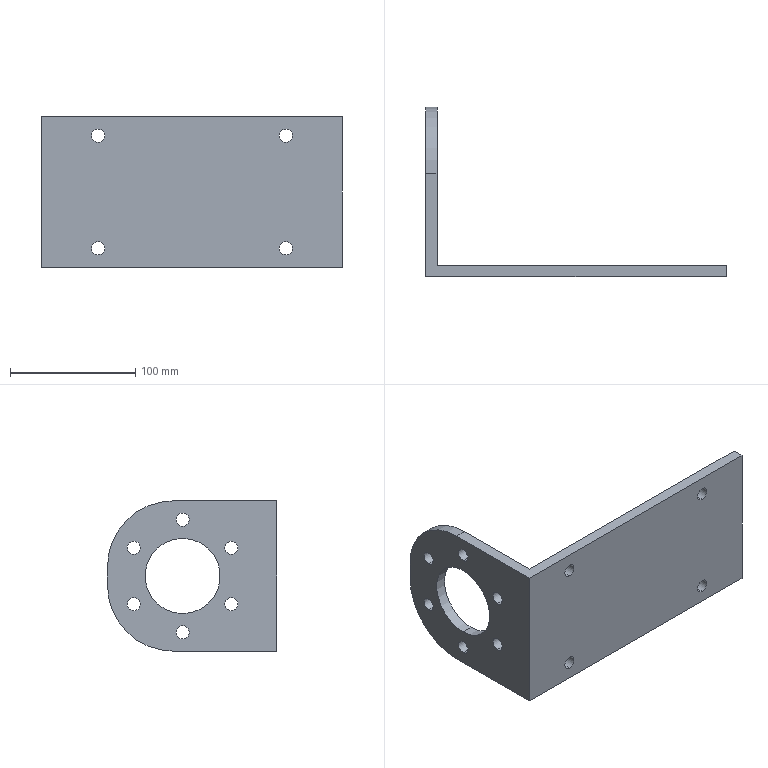Part | SolidWorks | features ICE 3, BaseBody 1 | 1 solid | 32 faces | box 240 x 135 x 120 mm | volume 351393 mm3 | cylinder 24 | plane 8 | commonest cylinder face diameters 10.5 x20 60 x2 105 x2
STEP:
#1=CARTESIAN_POINT('',(195.,9.,-39.75));
#2=VERTEX_POINT('',#1);
#3=CARTESIAN_POINT('',(195.,9.,-50.25));
#4=VERTEX_POINT('',#3);
#5=CARTESIAN_POINT('',(195.,9.,-45.));
#6=DIRECTION('',(0.,-1.,0.));
#7=DIRECTION('',(0.,0.,-1.));
#8=AXIS2_PLACEMENT_3D('',#5,#6,#7);
#9=CIRCLE('',#8,5.25);
#10=EDGE_CURVE('',#2,#4,#9,.T.);
#11=ORIENTED_EDGE('',*,*,#10,.F.);
#12=CARTESIAN_POINT('',(195.,0.,-39.75));
#13=VERTEX_POINT('',#12);
#14=CARTESIAN_POINT('',(195.,135.,-39.75));
#15=DIRECTION('',(0.,-1.,0.));
#16=VECTOR('',#15,1000.);
#17=LINE('',#14,#16);
#18=EDGE_CURVE('',#2,#13,#17,.T.);
#19=ORIENTED_EDGE('',*,*,#18,.T.);
#20=CARTESIAN_POINT('',(195.,0.,-50.25));
#21=VERTEX_POINT('',#20);
#22=CARTESIAN_POINT('',(195.,0.,-45.));
#23=DIRECTION('',(0.,-1.,0.));
#24=DIRECTION('',(0.,0.,-1.));
#25=AXIS2_PLACEMENT_3D('',#22,#23,#24);
#26=CIRCLE('',#25,5.25);
#27=EDGE_CURVE('',#13,#21,#26,.T.);
#28=ORIENTED_EDGE('',*,*,#27,.T.);
#29=CARTESIAN_POINT('',(195.,135.,-50.25));
#30=DIRECTION('',(0.,-1.,0.));
#31=VECTOR('',#30,1000.);
#32=LINE('',#29,#31);
#33=EDGE_CURVE('',#4,#21,#32,.T.);
#34=ORIENTED_EDGE('',*,*,#33,.F.);
#35=EDGE_LOOP('',(#11,#19,#28,#34));
#36=FACE_OUTER_BOUND('',#35,.T.);
#37=CARTESIAN_POINT('',(195.,135.,-45.));
#38=DIRECTION('',(0.,-1.,0.));
#39=DIRECTION('',(0.,0.,-1.));
#40=AXIS2_PLACEMENT_3D('',#37,#38,#39);
#41=CYLINDRICAL_SURFACE('',#40,5.25);
#42=ADVANCED_FACE('',(#36),#41,.F.);
#43=CARTESIAN_POINT('',(45.,9.,-39.75));
#44=VERTEX_POINT('',#43);
#45=CARTESIAN_POINT('',(45.,9.,-50.25));
#46=VERTEX_POINT('',#45);
#47=CARTESIAN_POINT('',(45.,9.,-45.));
#48=DIRECTION('',(0.,-1.,0.));
#49=DIRECTION('',(0.,0.,-1.));
#50=AXIS2_PLACEMENT_3D('',#47,#48,#49);
#51=CIRCLE('',#50,5.25);
#52=EDGE_CURVE('',#44,#46,#51,.T.);
#53=ORIENTED_EDGE('',*,*,#52,.F.);
#54=CARTESIAN_POINT('',(45.,0.,-39.75));
#55=VERTEX_POINT('',#54);
#56=CARTESIAN_POINT('',(45.,135.,-39.75));
#57=DIRECTION('',(0.,-1.,0.));
#58=VECTOR('',#57,1000.);
#59=LINE('',#56,#58);
#60=EDGE_CURVE('',#44,#55,#59,.T.);
#61=ORIENTED_EDGE('',*,*,#60,.T.);
#62=CARTESIAN_POINT('',(45.,0.,-50.25));
#63=VERTEX_POINT('',#62);
#64=CARTESIAN_POINT('',(45.,0.,-45.));
#65=DIRECTION('',(0.,-1.,0.));
#66=DIRECTION('',(0.,0.,-1.));
#67=AXIS2_PLACEMENT_3D('',#64,#65,#66);
#68=CIRCLE('',#67,5.25);
#69=EDGE_CURVE('',#55,#63,#68,.T.);
#70=ORIENTED_EDGE('',*,*,#69,.T.);
#71=CARTESIAN_POINT('',(45.,135.,-50.25));
#72=DIRECTION('',(0.,-1.,0.));
#73=VECTOR('',#72,1000.);
#74=LINE('',#71,#73);
#75=EDGE_CURVE('',#46,#63,#74,.T.);
#76=ORIENTED_EDGE('',*,*,#75,.F.);
#77=EDGE_LOOP('',(#53,#61,#70,#76));
#78=FACE_OUTER_BOUND('',#77,.T.);
#79=CARTESIAN_POINT('',(45.,135.,-45.));
#80=DIRECTION('',(0.,-1.,0.));
#81=DIRECTION('',(0.,0.,-1.));
#82=AXIS2_PLACEMENT_3D('',#79,#80,#81);
#83=CYLINDRICAL_SURFACE('',#82,5.25);
#84=ADVANCED_FACE('',(#78),#83,.F.);
#85=CARTESIAN_POINT('',(45.,9.,50.25));
#86=VERTEX_POINT('',#85);
#87=CARTESIAN_POINT('',(45.,9.,39.75));
#88=VERTEX_POINT('',#87);
#89=CARTESIAN_POINT('',(45.,9.,45.));
#90=DIRECTION('',(0.,-1.,0.));
#91=DIRECTION('',(0.,0.,-1.));
#92=AXIS2_PLACEMENT_3D('',#89,#90,#91);
#93=CIRCLE('',#92,5.25);
#94=EDGE_CURVE('',#86,#88,#93,.T.);
#95=ORIENTED_EDGE('',*,*,#94,.F.);
#96=CARTESIAN_POINT('',(45.,0.,50.25));
#97=VERTEX_POINT('',#96);
#98=CARTESIAN_POINT('',(45.,135.,50.25));
#99=DIRECTION('',(0.,-1.,0.));
#100=VECTOR('',#99,1000.);
#101=LINE('',#98,#100);
#102=EDGE_CURVE('',#86,#97,#101,.T.);
#103=ORIENTED_EDGE('',*,*,#102,.T.);
#104=CARTESIAN_POINT('',(45.,0.,39.75));
#105=VERTEX_POINT('',#104);
#106=CARTESIAN_POINT('',(45.,0.,45.));
#107=DIRECTION('',(0.,-1.,0.));
#108=DIRECTION('',(0.,0.,-1.));
#109=AXIS2_PLACEMENT_3D('',#106,#107,#108);
#110=CIRCLE('',#109,5.25);
#111=EDGE_CURVE('',#97,#105,#110,.T.);
#112=ORIENTED_EDGE('',*,*,#111,.T.);
#113=CARTESIAN_POINT('',(45.,135.,39.75));
#114=DIRECTION('',(0.,-1.,0.));
#115=VECTOR('',#114,1000.);
#116=LINE('',#113,#115);
#117=EDGE_CURVE('',#88,#105,#116,.T.);
#118=ORIENTED_EDGE('',*,*,#117,.F.);
#119=EDGE_LOOP('',(#95,#103,#112,#118));
#120=FACE_OUTER_BOUND('',#119,.T.);
#121=CARTESIAN_POINT('',(45.,135.,45.));
#122=DIRECTION('',(0.,-1.,0.));
#123=DIRECTION('',(0.,0.,-1.));
#124=AXIS2_PLACEMENT_3D('',#121,#122,#123);
#125=CYLINDRICAL_SURFACE('',#124,5.25);
#126=ADVANCED_FACE('',(#120),#125,.F.);
#127=CARTESIAN_POINT('',(195.,9.,50.25));
#128=VERTEX_POINT('',#127);
#129=CARTESIAN_POINT('',(195.,9.,39.75));
#130=VERTEX_POINT('',#129);
#131=CARTESIAN_POINT('',(195.,9.,45.));
#132=DIRECTION('',(0.,-1.,0.));
#133=DIRECTION('',(0.,0.,-1.));
#134=AXIS2_PLACEMENT_3D('',#131,#132,#133);
#135=CIRCLE('',#134,5.25);
#136=EDGE_CURVE('',#128,#130,#135,.T.);
#137=ORIENTED_EDGE('',*,*,#136,.F.);
#138=CARTESIAN_POINT('',(195.,0.,50.25));
#139=VERTEX_POINT('',#138);
#140=CARTESIAN_POINT('',(195.,135.,50.25));
#141=DIRECTION('',(0.,-1.,0.));
#142=VECTOR('',#141,1000.);
#143=LINE('',#140,#142);
#144=EDGE_CURVE('',#128,#139,#143,.T.);
#145=ORIENTED_EDGE('',*,*,#144,.T.);
#146=CARTESIAN_POINT('',(195.,0.,39.75));
#147=VERTEX_POINT('',#146);
#148=CARTESIAN_POINT('',(195.,0.,45.));
#149=DIRECTION('',(0.,-1.,0.));
#150=DIRECTION('',(0.,0.,-1.));
#151=AXIS2_PLACEMENT_3D('',#148,#149,#150);
#152=CIRCLE('',#151,5.25);
#153=EDGE_CURVE('',#139,#147,#152,.T.);
#154=ORIENTED_EDGE('',*,*,#153,.T.);
#155=CARTESIAN_POINT('',(195.,135.,39.75));
#156=DIRECTION('',(0.,-1.,0.));
#157=VECTOR('',#156,1000.);
#158=LINE('',#155,#157);
#159=EDGE_CURVE('',#130,#147,#158,.T.);
#160=ORIENTED_EDGE('',*,*,#159,.F.);
#161=EDGE_LOOP('',(#137,#145,#154,#160));
#162=FACE_OUTER_BOUND('',#161,.T.);
#163=CARTESIAN_POINT('',(195.,135.,45.));
#164=DIRECTION('',(0.,-1.,0.));
#165=DIRECTION('',(0.,0.,-1.));
#166=AXIS2_PLACEMENT_3D('',#163,#164,#165);
#167=CYLINDRICAL_SURFACE('',#166,5.25);
#168=ADVANCED_FACE('',(#162),#167,.F.);
#169=CARTESIAN_POINT('',(9.,75.,30.));
#170=VERTEX_POINT('',#169);
#171=CARTESIAN_POINT('',(9.,75.,-30.));
#172=VERTEX_POINT('',#171);
#173=CARTESIAN_POINT('',(9.,75.,0.));
#174=DIRECTION('',(1.,0.,0.));
#175=DIRECTION('',(0.,0.,1.));
#176=AXIS2_PLACEMENT_3D('',#173,#174,#175);
#177=CIRCLE('',#176,30.);
#178=EDGE_CURVE('',#170,#172,#177,.T.);
#179=ORIENTED_EDGE('',*,*,#178,.T.);
#180=CARTESIAN_POINT('',(0.,75.,-30.));
#181=VERTEX_POINT('',#180);
#182=CARTESIAN_POINT('',(9.,75.,-30.));
#183=DIRECTION('',(-1.,0.,0.));
#184=VECTOR('',#183,1000.);
#185=LINE('',#182,#184);
#186=EDGE_CURVE('',#172,#181,#185,.T.);
#187=ORIENTED_EDGE('',*,*,#186,.T.);
#188=CARTESIAN_POINT('',(0.,75.,30.));
#189=VERTEX_POINT('',#188);
#190=CARTESIAN_POINT('',(0.,75.,0.));
#191=DIRECTION('',(1.,0.,0.));
#192=DIRECTION('',(0.,0.,1.));
#193=AXIS2_PLACEMENT_3D('',#190,#191,#192);
#194=CIRCLE('',#193,30.);
#195=EDGE_CURVE('',#189,#181,#194,.T.);
#196=ORIENTED_EDGE('',*,*,#195,.F.);
#197=CARTESIAN_POINT('',(9.,75.,30.));
#198=DIRECTION('',(-1.,0.,0.));
#199=VECTOR('',#198,1000.);
#200=LINE('',#197,#199);
#201=EDGE_CURVE('',#170,#189,#200,.T.);
#202=ORIENTED_EDGE('',*,*,#201,.F.);
#203=EDGE_LOOP('',(#179,#187,#196,#202));
#204=FACE_OUTER_BOUND('',#203,.T.);
#205=CARTESIAN_POINT('',(9.,75.,0.));
#206=DIRECTION('',(-1.,0.,0.));
#207=DIRECTION('',(0.,0.,1.));
#208=AXIS2_PLACEMENT_3D('',#205,#206,#207);
#209=CYLINDRICAL_SURFACE('',#208,30.);
#210=ADVANCED_FACE('',(#204),#209,.F.);
#211=CARTESIAN_POINT('',(9.,75.,50.25));
#212=VERTEX_POINT('',#211);
#213=CARTESIAN_POINT('',(9.,75.,39.75));
#214=VERTEX_POINT('',#213);
#215=CARTESIAN_POINT('',(9.,75.,45.));
#216=DIRECTION('',(1.,0.,0.));
#217=DIRECTION('',(0.,0.,1.));
#218=AXIS2_PLACEMENT_3D('',#215,#216,#217);
#219=CIRCLE('',#218,5.25);
#220=EDGE_CURVE('',#212,#214,#219,.T.);
#221=ORIENTED_EDGE('',*,*,#220,.T.);
#222=CARTESIAN_POINT('',(0.,75.,39.75));
#223=VERTEX_POINT('',#222);
#224=CARTESIAN_POINT('',(9.,75.,39.75));
#225=DIRECTION('',(-1.,0.,0.));
#226=VECTOR('',#225,1000.);
#227=LINE('',#224,#226);
#228=EDGE_CURVE('',#214,#223,#227,.T.);
#229=ORIENTED_EDGE('',*,*,#228,.T.);
#230=CARTESIAN_POINT('',(0.,75.,50.25));
#231=VERTEX_POINT('',#230);
#232=CARTESIAN_POINT('',(0.,75.,45.));
#233=DIRECTION('',(1.,0.,0.));
#234=DIRECTION('',(0.,0.,1.));
#235=AXIS2_PLACEMENT_3D('',#232,#233,#234);
#236=CIRCLE('',#235,5.25);
#237=EDGE_CURVE('',#231,#223,#236,.T.);
#238=ORIENTED_EDGE('',*,*,#237,.F.);
#239=CARTESIAN_POINT('',(9.,75.,50.25));
#240=DIRECTION('',(-1.,0.,0.));
#241=VECTOR('',#240,1000.);
#242=LINE('',#239,#241);
#243=EDGE_CURVE('',#212,#231,#242,.T.);
#244=ORIENTED_EDGE('',*,*,#243,.F.);
#245=EDGE_LOOP('',(#221,#229,#238,#244));
#246=FACE_OUTER_BOUND('',#245,.T.);
#247=CARTESIAN_POINT('',(9.,75.,45.));
#248=DIRECTION('',(-1.,0.,0.));
#249=DIRECTION('',(0.,0.,1.));
#250=AXIS2_PLACEMENT_3D('',#247,#248,#249);
#251=CYLINDRICAL_SURFACE('',#250,5.25);
#252=ADVANCED_FACE('',(#246),#251,.F.);
#253=CARTESIAN_POINT('',(9.,113.971,27.75));
#254=VERTEX_POINT('',#253);
#255=CARTESIAN_POINT('',(9.,113.971,17.25));
#256=VERTEX_POINT('',#255);
#257=CARTESIAN_POINT('',(9.,113.971,22.5));
#258=DIRECTION('',(1.,0.,0.));
#259=DIRECTION('',(0.,0.,1.));
#260=AXIS2_PLACEMENT_3D('',#257,#258,#259);
#261=CIRCLE('',#260,5.25);
#262=EDGE_CURVE('',#254,#256,#261,.T.);
#263=ORIENTED_EDGE('',*,*,#262,.T.);
#264=CARTESIAN_POINT('',(0.,113.971,17.25));
#265=VERTEX_POINT('',#264);
#266=CARTESIAN_POINT('',(9.,113.971,17.25));
#267=DIRECTION('',(-1.,0.,0.));
#268=VECTOR('',#267,1000.);
#269=LINE('',#266,#268);
#270=EDGE_CURVE('',#256,#265,#269,.T.);
#271=ORIENTED_EDGE('',*,*,#270,.T.);
#272=CARTESIAN_POINT('',(0.,113.971,27.75));
#273=VERTEX_POINT('',#272);
#274=CARTESIAN_POINT('',(0.,113.971,22.5));
#275=DIRECTION('',(1.,0.,0.));
#276=DIRECTION('',(0.,0.,1.));
#277=AXIS2_PLACEMENT_3D('',#274,#275,#276);
#278=CIRCLE('',#277,5.25);
#279=EDGE_CURVE('',#273,#265,#278,.T.);
#280=ORIENTED_EDGE('',*,*,#279,.F.);
#281=CARTESIAN_POINT('',(9.,113.971,27.75));
#282=DIRECTION('',(-1.,0.,0.));
#283=VECTOR('',#282,1000.);
#284=LINE('',#281,#283);
#285=EDGE_CURVE('',#254,#273,#284,.T.);
#286=ORIENTED_EDGE('',*,*,#285,.F.);
#287=EDGE_LOOP('',(#263,#271,#280,#286));
#288=FACE_OUTER_BOUND('',#287,.T.);
#289=CARTESIAN_POINT('',(9.,113.971,22.5));
#290=DIRECTION('',(-1.,0.,0.));
#291=DIRECTION('',(0.,0.,1.));
#292=AXIS2_PLACEMENT_3D('',#289,#290,#291);
#293=CYLINDRICAL_SURFACE('',#292,5.25);
#294=ADVANCED_FACE('',(#288),#293,.F.);
#295=CARTESIAN_POINT('',(9.,113.971,-17.25));
#296=VERTEX_POINT('',#295);
#297=CARTESIAN_POINT('',(9.,113.971,-27.75));
#298=VERTEX_POINT('',#297);
#299=CARTESIAN_POINT('',(9.,113.971,-22.5));
#300=DIRECTION('',(1.,0.,0.));
#301=DIRECTION('',(0.,0.,1.));
#302=AXIS2_PLACEMENT_3D('',#299,#300,#301);
#303=CIRCLE('',#302,5.25);
#304=EDGE_CURVE('',#296,#298,#303,.T.);
#305=ORIENTED_EDGE('',*,*,#304,.T.);
#306=CARTESIAN_POINT('',(0.,113.971,-27.75));
#307=VERTEX_POINT('',#306);
#308=CARTESIAN_POINT('',(9.,113.971,-27.75));
#309=DIRECTION('',(-1.,0.,0.));
#310=VECTOR('',#309,1000.);
#311=LINE('',#308,#310);
#312=EDGE_CURVE('',#298,#307,#311,.T.);
#313=ORIENTED_EDGE('',*,*,#312,.T.);
#314=CARTESIAN_POINT('',(0.,113.971,-17.25));
#315=VERTEX_POINT('',#314);
#316=CARTESIAN_POINT('',(0.,113.971,-22.5));
#317=DIRECTION('',(1.,0.,0.));
#318=DIRECTION('',(0.,0.,1.));
#319=AXIS2_PLACEMENT_3D('',#316,#317,#318);
#320=CIRCLE('',#319,5.25);
#321=EDGE_CURVE('',#315,#307,#320,.T.);
#322=ORIENTED_EDGE('',*,*,#321,.F.);
#323=CARTESIAN_POINT('',(9.,113.971,-17.25));
#324=DIRECTION('',(-1.,0.,0.));
#325=VECTOR('',#324,1000.);
#326=LINE('',#323,#325);
#327=EDGE_CURVE('',#296,#315,#326,.T.);
#328=ORIENTED_EDGE('',*,*,#327,.F.);
#329=EDGE_LOOP('',(#305,#313,#322,#328));
#330=FACE_OUTER_BOUND('',#329,.T.);
#331=CARTESIAN_POINT('',(9.,113.971,-22.5));
#332=DIRECTION('',(-1.,0.,0.));
#333=DIRECTION('',(0.,0.,1.));
#334=AXIS2_PLACEMENT_3D('',#331,#332,#333);
#335=CYLINDRICAL_SURFACE('',#334,5.25);
#336=ADVANCED_FACE('',(#330),#335,.F.);
#337=CARTESIAN_POINT('',(9.,75.,-39.75));
#338=VERTEX_POINT('',#337);
#339=CARTESIAN_POINT('',(9.,75.,-50.25));
#340=VERTEX_POINT('',#339);
#341=CARTESIAN_POINT('',(9.,75.,-45.));
#342=DIRECTION('',(1.,0.,0.));
#343=DIRECTION('',(0.,0.,1.));
#344=AXIS2_PLACEMENT_3D('',#341,#342,#343);
#345=CIRCLE('',#344,5.25);
#346=EDGE_CURVE('',#338,#340,#345,.T.);
#347=ORIENTED_EDGE('',*,*,#346,.T.);
#348=CARTESIAN_POINT('',(0.,75.,-50.25));
#349=VERTEX_POINT('',#348);
#350=CARTESIAN_POINT('',(9.,75.,-50.25));
#351=DIRECTION('',(-1.,0.,0.));
#352=VECTOR('',#351,1000.);
#353=LINE('',#350,#352);
#354=EDGE_CURVE('',#340,#349,#353,.T.);
#355=ORIENTED_EDGE('',*,*,#354,.T.);
#356=CARTESIAN_POINT('',(0.,75.,-39.75));
#357=VERTEX_POINT('',#356);
#358=CARTESIAN_POINT('',(0.,75.,-45.));
#359=DIRECTION('',(1.,0.,0.));
#360=DIRECTION('',(0.,0.,1.));
#361=AXIS2_PLACEMENT_3D('',#358,#359,#360);
#362=CIRCLE('',#361,5.25);
#363=EDGE_CURVE('',#357,#349,#362,.T.);
#364=ORIENTED_EDGE('',*,*,#363,.F.);
#365=CARTESIAN_POINT('',(9.,75.,-39.75));
#366=DIRECTION('',(-1.,0.,0.));
#367=VECTOR('',#366,1000.);
#368=LINE('',#365,#367);
#369=EDGE_CURVE('',#338,#357,#368,.T.);
#370=ORIENTED_EDGE('',*,*,#369,.F.);
#371=EDGE_LOOP('',(#347,#355,#364,#370));
#372=FACE_OUTER_BOUND('',#371,.T.);
#373=CARTESIAN_POINT('',(9.,75.,-45.));
#374=DIRECTION('',(-1.,0.,0.));
#375=DIRECTION('',(0.,0.,1.));
#376=AXIS2_PLACEMENT_3D('',#373,#374,#375);
#377=CYLINDRICAL_SURFACE('',#376,5.25);
#378=ADVANCED_FACE('',(#372),#377,.F.);
#379=CARTESIAN_POINT('',(9.,36.029,-17.25));
#380=VERTEX_POINT('',#379);
#381=CARTESIAN_POINT('',(9.,36.029,-27.75));
#382=VERTEX_POINT('',#381);
#383=CARTESIAN_POINT('',(9.,36.029,-22.5));
#384=DIRECTION('',(1.,0.,0.));
#385=DIRECTION('',(0.,0.,1.));
#386=AXIS2_PLACEMENT_3D('',#383,#384,#385);
#387=CIRCLE('',#386,5.25);
#388=EDGE_CURVE('',#380,#382,#387,.T.);
#389=ORIENTED_EDGE('',*,*,#388,.T.);
#390=CARTESIAN_POINT('',(0.,36.029,-27.75));
#391=VERTEX_POINT('',#390);
#392=CARTESIAN_POINT('',(9.,36.029,-27.75));
#393=DIRECTION('',(-1.,0.,0.));
#394=VECTOR('',#393,1000.);
#395=LINE('',#392,#394);
#396=EDGE_CURVE('',#382,#391,#395,.T.);
#397=ORIENTED_EDGE('',*,*,#396,.T.);
#398=CARTESIAN_POINT('',(0.,36.029,-17.25));
#399=VERTEX_POINT('',#398);
#400=CARTESIAN_POINT('',(0.,36.029,-22.5));
#401=DIRECTION('',(1.,0.,0.));
#402=DIRECTION('',(0.,0.,1.));
#403=AXIS2_PLACEMENT_3D('',#400,#401,#402);
#404=CIRCLE('',#403,5.25);
#405=EDGE_CURVE('',#399,#391,#404,.T.);
#406=ORIENTED_EDGE('',*,*,#405,.F.);
#407=CARTESIAN_POINT('',(9.,36.029,-17.25));
#408=DIRECTION('',(-1.,0.,0.));
#409=VECTOR('',#408,1000.);
#410=LINE('',#407,#409);
#411=EDGE_CURVE('',#380,#399,#410,.T.);
#412=ORIENTED_EDGE('',*,*,#411,.F.);
#413=EDGE_LOOP('',(#389,#397,#406,#412));
#414=FACE_OUTER_BOUND('',#413,.T.);
#415=CARTESIAN_POINT('',(9.,36.029,-22.5));
#416=DIRECTION('',(-1.,0.,0.));
#417=DIRECTION('',(0.,0.,1.));
#418=AXIS2_PLACEMENT_3D('',#415,#416,#417);
#419=CYLINDRICAL_SURFACE('',#418,5.25);
#420=ADVANCED_FACE('',(#414),#419,.F.);
#421=CARTESIAN_POINT('',(9.,36.029,27.75));
#422=VERTEX_POINT('',#421);
#423=CARTESIAN_POINT('',(9.,36.029,17.25));
#424=VERTEX_POINT('',#423);
#425=CARTESIAN_POINT('',(9.,36.029,22.5));
#426=DIRECTION('',(1.,0.,0.));
#427=DIRECTION('',(0.,0.,1.));
#428=AXIS2_PLACEMENT_3D('',#425,#426,#427);
#429=CIRCLE('',#428,5.25);
#430=EDGE_CURVE('',#422,#424,#429,.T.);
#431=ORIENTED_EDGE('',*,*,#430,.T.);
#432=CARTESIAN_POINT('',(0.,36.029,17.25));
#433=VERTEX_POINT('',#432);
#434=CARTESIAN_POINT('',(9.,36.029,17.25));
#435=DIRECTION('',(-1.,0.,0.));
#436=VECTOR('',#435,1000.);
#437=LINE('',#434,#436);
#438=EDGE_CURVE('',#424,#433,#437,.T.);
#439=ORIENTED_EDGE('',*,*,#438,.T.);
#440=CARTESIAN_POINT('',(0.,36.029,27.75));
#441=VERTEX_POINT('',#440);
#442=CARTESIAN_POINT('',(0.,36.029,22.5));
#443=DIRECTION('',(1.,0.,0.));
#444=DIRECTION('',(0.,0.,1.));
#445=AXIS2_PLACEMENT_3D('',#442,#443,#444);
#446=CIRCLE('',#445,5.25);
#447=EDGE_CURVE('',#441,#433,#446,.T.);
#448=ORIENTED_EDGE('',*,*,#447,.F.);
#449=CARTESIAN_POINT('',(9.,36.029,27.75));
#450=DIRECTION('',(-1.,0.,0.));
#451=VECTOR('',#450,1000.);
#452=LINE('',#449,#451);
#453=EDGE_CURVE('',#422,#441,#452,.T.);
#454=ORIENTED_EDGE('',*,*,#453,.F.);
#455=EDGE_LOOP('',(#431,#439,#448,#454));
#456=FACE_OUTER_BOUND('',#455,.T.);
#457=CARTESIAN_POINT('',(9.,36.029,22.5));
#458=DIRECTION('',(-1.,0.,0.));
#459=DIRECTION('',(0.,0.,1.));
#460=AXIS2_PLACEMENT_3D('',#457,#458,#459);
#461=CYLINDRICAL_SURFACE('',#460,5.25);
#462=ADVANCED_FACE('',(#456),#461,.F.);
#463=CARTESIAN_POINT('',(195.,0.,-45.));
#464=DIRECTION('',(0.,-1.,0.));
#465=DIRECTION('',(0.,0.,-1.));
#466=AXIS2_PLACEMENT_3D('',#463,#464,#465);
#467=CIRCLE('',#466,5.25);
#468=EDGE_CURVE('',#21,#13,#467,.T.);
#469=ORIENTED_EDGE('',*,*,#468,.F.);
#470=ORIENTED_EDGE('',*,*,#27,.F.);
#471=EDGE_LOOP('',(#469,#470));
#472=FACE_BOUND('',#471,.T.);
#473=CARTESIAN_POINT('',(45.,0.,-45.));
#474=DIRECTION('',(0.,-1.,0.));
#475=DIRECTION('',(0.,0.,-1.));
#476=AXIS2_PLACEMENT_3D('',#473,#474,#475);
#477=CIRCLE('',#476,5.25);
#478=EDGE_CURVE('',#63,#55,#477,.T.);
#479=ORIENTED_EDGE('',*,*,#478,.F.);
#480=ORIENTED_EDGE('',*,*,#69,.F.);
#481=EDGE_LOOP('',(#479,#480));
#482=FACE_BOUND('',#481,.T.);
#483=CARTESIAN_POINT('',(45.,0.,45.));
#484=DIRECTION('',(0.,-1.,0.));
#485=DIRECTION('',(0.,0.,-1.));
#486=AXIS2_PLACEMENT_3D('',#483,#484,#485);
#487=CIRCLE('',#486,5.25);
#488=EDGE_CURVE('',#105,#97,#487,.T.);
#489=ORIENTED_EDGE('',*,*,#488,.F.);
#490=ORIENTED_EDGE('',*,*,#111,.F.);
#491=EDGE_LOOP('',(#489,#490));
#492=FACE_BOUND('',#491,.T.);
#493=CARTESIAN_POINT('',(195.,0.,45.));
#494=DIRECTION('',(0.,-1.,0.));
#495=DIRECTION('',(0.,0.,-1.));
#496=AXIS2_PLACEMENT_3D('',#493,#494,#495);
#497=CIRCLE('',#496,5.25);
#498=EDGE_CURVE('',#147,#139,#497,.T.);
#499=ORIENTED_EDGE('',*,*,#498,.F.);
#500=ORIENTED_EDGE('',*,*,#153,.F.);
#501=EDGE_LOOP('',(#499,#500));
#502=FACE_BOUND('',#501,.T.);
#503=CARTESIAN_POINT('',(240.,0.,60.));
#504=VERTEX_POINT('',#503);
#505=CARTESIAN_POINT('',(0.,0.,60.));
#506=VERTEX_POINT('',#505);
#507=CARTESIAN_POINT('',(52.5,0.,60.));
#508=DIRECTION('',(-1.,0.,0.));
#509=VECTOR('',#508,1000.);
#510=LINE('',#507,#509);
#511=EDGE_CURVE('',#504,#506,#510,.T.);
#512=ORIENTED_EDGE('',*,*,#511,.T.);
#513=CARTESIAN_POINT('',(0.,0.,-60.));
#514=VERTEX_POINT('',#513);
#515=CARTESIAN_POINT('',(0.,0.,0.));
#516=DIRECTION('',(0.,0.,-1.));
#517=VECTOR('',#516,1000.);
#518=LINE('',#515,#517);
#519=EDGE_CURVE('',#506,#514,#518,.T.);
#520=ORIENTED_EDGE('',*,*,#519,.T.);
#521=CARTESIAN_POINT('',(240.,0.,-60.));
#522=VERTEX_POINT('',#521);
#523=CARTESIAN_POINT('',(52.5,0.,-60.));
#524=DIRECTION('',(1.,0.,0.));
#525=VECTOR('',#524,1000.);
#526=LINE('',#523,#525);
#527=EDGE_CURVE('',#514,#522,#526,.T.);
#528=ORIENTED_EDGE('',*,*,#527,.T.);
#529=CARTESIAN_POINT('',(240.,0.,60.));
#530=DIRECTION('',(0.,0.,-1.));
#531=VECTOR('',#530,1000.);
#532=LINE('',#529,#531);
#533=EDGE_CURVE('',#504,#522,#532,.T.);
#534=ORIENTED_EDGE('',*,*,#533,.F.);
#535=EDGE_LOOP('',(#512,#520,#528,#534));
#536=FACE_OUTER_BOUND('',#535,.T.);
#537=CARTESIAN_POINT('',(0.,0.,60.));
#538=DIRECTION('',(0.,-1.,0.));
#539=DIRECTION('',(0.,0.,-1.));
#540=AXIS2_PLACEMENT_3D('',#537,#538,#539);
#541=PLANE('',#540);
#542=ADVANCED_FACE('',(#472,#482,#492,#502,#536),#541,.T.);
#543=CARTESIAN_POINT('',(195.,9.,-45.));
#544=DIRECTION('',(0.,-1.,0.));
#545=DIRECTION('',(0.,0.,-1.));
#546=AXIS2_PLACEMENT_3D('',#543,#544,#545);
#547=CIRCLE('',#546,5.25);
#548=EDGE_CURVE('',#4,#2,#547,.T.);
#549=ORIENTED_EDGE('',*,*,#548,.T.);
#550=ORIENTED_EDGE('',*,*,#10,.T.);
#551=EDGE_LOOP('',(#549,#550));
#552=FACE_BOUND('',#551,.T.);
#553=CARTESIAN_POINT('',(45.,9.,-45.));
#554=DIRECTION('',(0.,-1.,0.));
#555=DIRECTION('',(0.,0.,-1.));
#556=AXIS2_PLACEMENT_3D('',#553,#554,#555);
#557=CIRCLE('',#556,5.25);
#558=EDGE_CURVE('',#46,#44,#557,.T.);
#559=ORIENTED_EDGE('',*,*,#558,.T.);
#560=ORIENTED_EDGE('',*,*,#52,.T.);
#561=EDGE_LOOP('',(#559,#560));
#562=FACE_BOUND('',#561,.T.);
#563=CARTESIAN_POINT('',(45.,9.,45.));
#564=DIRECTION('',(0.,-1.,0.));
#565=DIRECTION('',(0.,0.,-1.));
#566=AXIS2_PLACEMENT_3D('',#563,#564,#565);
#567=CIRCLE('',#566,5.25);
#568=EDGE_CURVE('',#88,#86,#567,.T.);
#569=ORIENTED_EDGE('',*,*,#568,.T.);
#570=ORIENTED_EDGE('',*,*,#94,.T.);
#571=EDGE_LOOP('',(#569,#570));
#572=FACE_BOUND('',#571,.T.);
#573=CARTESIAN_POINT('',(195.,9.,45.));
#574=DIRECTION('',(0.,-1.,0.));
#575=DIRECTION('',(0.,0.,-1.));
#576=AXIS2_PLACEMENT_3D('',#573,#574,#575);
#577=CIRCLE('',#576,5.25);
#578=EDGE_CURVE('',#130,#128,#577,.T.);
#579=ORIENTED_EDGE('',*,*,#578,.T.);
#580=ORIENTED_EDGE('',*,*,#136,.T.);
#581=EDGE_LOOP('',(#579,#580));
#582=FACE_BOUND('',#581,.T.);
#583=CARTESIAN_POINT('',(240.,9.,60.));
#584=VERTEX_POINT('',#583);
#585=CARTESIAN_POINT('',(9.,9.,60.));
#586=VERTEX_POINT('',#585);
#587=CARTESIAN_POINT('',(57.,9.,60.));
#588=DIRECTION('',(-1.,0.,0.));
#589=VECTOR('',#588,1000.);
#590=LINE('',#587,#589);
#591=EDGE_CURVE('',#584,#586,#590,.T.);
#592=ORIENTED_EDGE('',*,*,#591,.F.);
#593=CARTESIAN_POINT('',(240.,9.,-60.));
#594=VERTEX_POINT('',#593);
#595=CARTESIAN_POINT('',(240.,9.,-60.));
#596=DIRECTION('',(0.,0.,1.));
#597=VECTOR('',#596,1000.);
#598=LINE('',#595,#597);
#599=EDGE_CURVE('',#594,#584,#598,.T.);
#600=ORIENTED_EDGE('',*,*,#599,.F.);
#601=CARTESIAN_POINT('',(9.,9.,-60.));
#602=VERTEX_POINT('',#601);
#603=CARTESIAN_POINT('',(57.,9.,-60.));
#604=DIRECTION('',(1.,0.,0.));
#605=VECTOR('',#604,1000.);
#606=LINE('',#603,#605);
#607=EDGE_CURVE('',#602,#594,#606,.T.);
#608=ORIENTED_EDGE('',*,*,#607,.F.);
#609=CARTESIAN_POINT('',(9.,9.,0.));
#610=DIRECTION('',(0.,0.,-1.));
#611=VECTOR('',#610,1000.);
#612=LINE('',#609,#611);
#613=EDGE_CURVE('',#586,#602,#612,.T.);
#614=ORIENTED_EDGE('',*,*,#613,.F.);
#615=EDGE_LOOP('',(#592,#600,#608,#614));
#616=FACE_OUTER_BOUND('',#615,.T.);
#617=CARTESIAN_POINT('',(9.,9.,60.));
#618=DIRECTION('',(0.,-1.,0.));
#619=DIRECTION('',(0.,0.,-1.));
#620=AXIS2_PLACEMENT_3D('',#617,#618,#619);
#621=PLANE('',#620);
#622=ADVANCED_FACE('',(#552,#562,#572,#582,#616),#621,.F.);
#623=ORIENTED_EDGE('',*,*,#195,.T.);
#624=CARTESIAN_POINT('',(0.,75.,0.));
#625=DIRECTION('',(1.,0.,0.));
#626=DIRECTION('',(0.,0.,1.));
#627=AXIS2_PLACEMENT_3D('',#624,#625,#626);
#628=CIRCLE('',#627,30.);
#629=EDGE_CURVE('',#181,#189,#628,.T.);
#630=ORIENTED_EDGE('',*,*,#629,.T.);
#631=EDGE_LOOP('',(#623,#630));
#632=FACE_BOUND('',#631,.T.);
#633=ORIENTED_EDGE('',*,*,#237,.T.);
#634=CARTESIAN_POINT('',(0.,75.,45.));
#635=DIRECTION('',(1.,0.,0.));
#636=DIRECTION('',(0.,0.,1.));
#637=AXIS2_PLACEMENT_3D('',#634,#635,#636);
#638=CIRCLE('',#637,5.25);
#639=EDGE_CURVE('',#223,#231,#638,.T.);
#640=ORIENTED_EDGE('',*,*,#639,.T.);
#641=EDGE_LOOP('',(#633,#640));
#642=FACE_BOUND('',#641,.T.);
#643=ORIENTED_EDGE('',*,*,#279,.T.);
#644=CARTESIAN_POINT('',(0.,113.971,22.5));
#645=DIRECTION('',(1.,0.,0.));
#646=DIRECTION('',(0.,0.,1.));
#647=AXIS2_PLACEMENT_3D('',#644,#645,#646);
#648=CIRCLE('',#647,5.25);
#649=EDGE_CURVE('',#265,#273,#648,.T.);
#650=ORIENTED_EDGE('',*,*,#649,.T.);
#651=EDGE_LOOP('',(#643,#650));
#652=FACE_BOUND('',#651,.T.);
#653=ORIENTED_EDGE('',*,*,#321,.T.);
#654=CARTESIAN_POINT('',(0.,113.971,-22.5));
#655=DIRECTION('',(1.,0.,0.));
#656=DIRECTION('',(0.,0.,1.));
#657=AXIS2_PLACEMENT_3D('',#654,#655,#656);
#658=CIRCLE('',#657,5.25);
#659=EDGE_CURVE('',#307,#315,#658,.T.);
#660=ORIENTED_EDGE('',*,*,#659,.T.);
#661=EDGE_LOOP('',(#653,#660));
#662=FACE_BOUND('',#661,.T.);
#663=ORIENTED_EDGE('',*,*,#363,.T.);
#664=CARTESIAN_POINT('',(0.,75.,-45.));
#665=DIRECTION('',(1.,0.,0.));
#666=DIRECTION('',(0.,0.,1.));
#667=AXIS2_PLACEMENT_3D('',#664,#665,#666);
#668=CIRCLE('',#667,5.25);
#669=EDGE_CURVE('',#349,#357,#668,.T.);
#670=ORIENTED_EDGE('',*,*,#669,.T.);
#671=EDGE_LOOP('',(#663,#670));
#672=FACE_BOUND('',#671,.T.);
#673=ORIENTED_EDGE('',*,*,#405,.T.);
#674=CARTESIAN_POINT('',(0.,36.029,-22.5));
#675=DIRECTION('',(1.,0.,0.));
#676=DIRECTION('',(0.,0.,1.));
#677=AXIS2_PLACEMENT_3D('',#674,#675,#676);
#678=CIRCLE('',#677,5.25);
#679=EDGE_CURVE('',#391,#399,#678,.T.);
#680=ORIENTED_EDGE('',*,*,#679,.T.);
#681=EDGE_LOOP('',(#673,#680));
#682=FACE_BOUND('',#681,.T.);
#683=ORIENTED_EDGE('',*,*,#447,.T.);
#684=CARTESIAN_POINT('',(0.,36.029,22.5));
#685=DIRECTION('',(1.,0.,0.));
#686=DIRECTION('',(0.,0.,1.));
#687=AXIS2_PLACEMENT_3D('',#684,#685,#686);
#688=CIRCLE('',#687,5.25);
#689=EDGE_CURVE('',#433,#441,#688,.T.);
#690=ORIENTED_EDGE('',*,*,#689,.T.);
#691=EDGE_LOOP('',(#683,#690));
#692=FACE_BOUND('',#691,.T.);
#693=CARTESIAN_POINT('',(0.,135.,7.5));
#694=VERTEX_POINT('',#693);
#695=CARTESIAN_POINT('',(0.,135.,-7.5));
#696=VERTEX_POINT('',#695);
#697=CARTESIAN_POINT('',(0.,135.,0.));
#698=DIRECTION('',(0.,0.,-1.));
#699=VECTOR('',#698,1000.);
#700=LINE('',#697,#699);
#701=EDGE_CURVE('',#694,#696,#700,.T.);
#702=ORIENTED_EDGE('',*,*,#701,.T.);
#703=CARTESIAN_POINT('',(0.,82.5,-60.));
#704=VERTEX_POINT('',#703);
#705=CARTESIAN_POINT('',(0.,82.5,-7.5));
#706=DIRECTION('',(-1.,0.,0.));
#707=DIRECTION('',(0.,0.,-1.));
#708=AXIS2_PLACEMENT_3D('',#705,#706,#707);
#709=CIRCLE('',#708,52.5);
#710=EDGE_CURVE('',#696,#704,#709,.T.);
#711=ORIENTED_EDGE('',*,*,#710,.T.);
#712=CARTESIAN_POINT('',(0.,67.5,-60.));
#713=DIRECTION('',(0.,-1.,0.));
#714=VECTOR('',#713,1000.);
#715=LINE('',#712,#714);
#716=EDGE_CURVE('',#704,#514,#715,.T.);
#717=ORIENTED_EDGE('',*,*,#716,.T.);
#718=ORIENTED_EDGE('',*,*,#519,.F.);
#719=CARTESIAN_POINT('',(0.,82.5,60.));
#720=VERTEX_POINT('',#719);
#721=CARTESIAN_POINT('',(0.,67.5,60.));
#722=DIRECTION('',(0.,1.,0.));
#723=VECTOR('',#722,1000.);
#724=LINE('',#721,#723);
#725=EDGE_CURVE('',#506,#720,#724,.T.);
#726=ORIENTED_EDGE('',*,*,#725,.T.);
#727=CARTESIAN_POINT('',(0.,82.5,7.5));
#728=DIRECTION('',(-1.,0.,0.));
#729=DIRECTION('',(0.,0.,1.));
#730=AXIS2_PLACEMENT_3D('',#727,#728,#729);
#731=CIRCLE('',#730,52.5);
#732=EDGE_CURVE('',#720,#694,#731,.T.);
#733=ORIENTED_EDGE('',*,*,#732,.T.);
#734=EDGE_LOOP('',(#702,#711,#717,#718,#726,#733));
#735=FACE_OUTER_BOUND('',#734,.T.);
#736=CARTESIAN_POINT('',(0.,0.,-60.));
#737=DIRECTION('',(-1.,0.,0.));
#738=DIRECTION('',(0.,0.,1.));
#739=AXIS2_PLACEMENT_3D('',#736,#737,#738);
#740=PLANE('',#739);
#741=ADVANCED_FACE('',(#632,#642,#652,#662,#672,#682,#692,#735),#740,.T.);
#742=ORIENTED_EDGE('',*,*,#511,.F.);
#743=CARTESIAN_POINT('',(240.,9.,60.));
#744=DIRECTION('',(0.,-1.,0.));
#745=VECTOR('',#744,1000.);
#746=LINE('',#743,#745);
#747=EDGE_CURVE('',#584,#504,#746,.T.);
#748=ORIENTED_EDGE('',*,*,#747,.F.);
#749=ORIENTED_EDGE('',*,*,#591,.T.);
#750=CARTESIAN_POINT('',(9.,82.5,60.));
#751=VERTEX_POINT('',#750);
#752=CARTESIAN_POINT('',(9.,41.25,60.));
#753=DIRECTION('',(0.,-1.,0.));
#754=VECTOR('',#753,1000.);
#755=LINE('',#752,#754);
#756=EDGE_CURVE('',#751,#586,#755,.T.);
#757=ORIENTED_EDGE('',*,*,#756,.F.);
#758=CARTESIAN_POINT('',(52.5,82.5,60.));
#759=DIRECTION('',(1.,0.,0.));
#760=VECTOR('',#759,1000.);
#761=LINE('',#758,#760);
#762=EDGE_CURVE('',#720,#751,#761,.T.);
#763=ORIENTED_EDGE('',*,*,#762,.F.);
#764=ORIENTED_EDGE('',*,*,#725,.F.);
#765=EDGE_LOOP('',(#742,#748,#749,#757,#763,#764));
#766=FACE_OUTER_BOUND('',#765,.T.);
#767=CARTESIAN_POINT('',(105.,0.,60.));
#768=DIRECTION('',(0.,0.,-1.));
#769=DIRECTION('',(-1.,0.,0.));
#770=AXIS2_PLACEMENT_3D('',#767,#768,#769);
#771=PLANE('',#770);
#772=ADVANCED_FACE('',(#766),#771,.F.);
#773=ORIENTED_EDGE('',*,*,#716,.F.);
#774=CARTESIAN_POINT('',(9.,82.5,-60.));
#775=VERTEX_POINT('',#774);
#776=CARTESIAN_POINT('',(52.5,82.5,-60.));
#777=DIRECTION('',(1.,0.,0.));
#778=VECTOR('',#777,1000.);
#779=LINE('',#776,#778);
#780=EDGE_CURVE('',#704,#775,#779,.T.);
#781=ORIENTED_EDGE('',*,*,#780,.T.);
#782=CARTESIAN_POINT('',(9.,41.25,-60.));
#783=DIRECTION('',(0.,-1.,0.));
#784=VECTOR('',#783,1000.);
#785=LINE('',#782,#784);
#786=EDGE_CURVE('',#775,#602,#785,.T.);
#787=ORIENTED_EDGE('',*,*,#786,.T.);
#788=ORIENTED_EDGE('',*,*,#607,.T.);
#789=CARTESIAN_POINT('',(240.,0.,-60.));
#790=DIRECTION('',(0.,1.,0.));
#791=VECTOR('',#790,1000.);
#792=LINE('',#789,#791);
#793=EDGE_CURVE('',#522,#594,#792,.T.);
#794=ORIENTED_EDGE('',*,*,#793,.F.);
#795=ORIENTED_EDGE('',*,*,#527,.F.);
#796=EDGE_LOOP('',(#773,#781,#787,#788,#794,#795));
#797=FACE_OUTER_BOUND('',#796,.T.);
#798=CARTESIAN_POINT('',(105.,0.,-60.));
#799=DIRECTION('',(0.,0.,-1.));
#800=DIRECTION('',(-1.,0.,0.));
#801=AXIS2_PLACEMENT_3D('',#798,#799,#800);
#802=PLANE('',#801);
#803=ADVANCED_FACE('',(#797),#802,.T.);
#804=ORIENTED_EDGE('',*,*,#178,.F.);
#805=CARTESIAN_POINT('',(9.,75.,0.));
#806=DIRECTION('',(1.,0.,0.));
#807=DIRECTION('',(0.,0.,1.));
#808=AXIS2_PLACEMENT_3D('',#805,#806,#807);
#809=CIRCLE('',#808,30.);
#810=EDGE_CURVE('',#172,#170,#809,.T.);
#811=ORIENTED_EDGE('',*,*,#810,.F.);
#812=EDGE_LOOP('',(#804,#811));
#813=FACE_BOUND('',#812,.T.);
#814=ORIENTED_EDGE('',*,*,#220,.F.);
#815=CARTESIAN_POINT('',(9.,75.,45.));
#816=DIRECTION('',(1.,0.,0.));
#817=DIRECTION('',(0.,0.,1.));
#818=AXIS2_PLACEMENT_3D('',#815,#816,#817);
#819=CIRCLE('',#818,5.25);
#820=EDGE_CURVE('',#214,#212,#819,.T.);
#821=ORIENTED_EDGE('',*,*,#820,.F.);
#822=EDGE_LOOP('',(#814,#821));
#823=FACE_BOUND('',#822,.T.);
#824=ORIENTED_EDGE('',*,*,#262,.F.);
#825=CARTESIAN_POINT('',(9.,113.971,22.5));
#826=DIRECTION('',(1.,0.,0.));
#827=DIRECTION('',(0.,0.,1.));
#828=AXIS2_PLACEMENT_3D('',#825,#826,#827);
#829=CIRCLE('',#828,5.25);
#830=EDGE_CURVE('',#256,#254,#829,.T.);
#831=ORIENTED_EDGE('',*,*,#830,.F.);
#832=EDGE_LOOP('',(#824,#831));
#833=FACE_BOUND('',#832,.T.);
#834=ORIENTED_EDGE('',*,*,#304,.F.);
#835=CARTESIAN_POINT('',(9.,113.971,-22.5));
#836=DIRECTION('',(1.,0.,0.));
#837=DIRECTION('',(0.,0.,1.));
#838=AXIS2_PLACEMENT_3D('',#835,#836,#837);
#839=CIRCLE('',#838,5.25);
#840=EDGE_CURVE('',#298,#296,#839,.T.);
#841=ORIENTED_EDGE('',*,*,#840,.F.);
#842=EDGE_LOOP('',(#834,#841));
#843=FACE_BOUND('',#842,.T.);
#844=ORIENTED_EDGE('',*,*,#346,.F.);
#845=CARTESIAN_POINT('',(9.,75.,-45.));
#846=DIRECTION('',(1.,0.,0.));
#847=DIRECTION('',(0.,0.,1.));
#848=AXIS2_PLACEMENT_3D('',#845,#846,#847);
#849=CIRCLE('',#848,5.25);
#850=EDGE_CURVE('',#340,#338,#849,.T.);
#851=ORIENTED_EDGE('',*,*,#850,.F.);
#852=EDGE_LOOP('',(#844,#851));
#853=FACE_BOUND('',#852,.T.);
#854=ORIENTED_EDGE('',*,*,#388,.F.);
#855=CARTESIAN_POINT('',(9.,36.029,-22.5));
#856=DIRECTION('',(1.,0.,0.));
#857=DIRECTION('',(0.,0.,1.));
#858=AXIS2_PLACEMENT_3D('',#855,#856,#857);
#859=CIRCLE('',#858,5.25);
#860=EDGE_CURVE('',#382,#380,#859,.T.);
#861=ORIENTED_EDGE('',*,*,#860,.F.);
#862=EDGE_LOOP('',(#854,#861));
#863=FACE_BOUND('',#862,.T.);
#864=ORIENTED_EDGE('',*,*,#430,.F.);
#865=CARTESIAN_POINT('',(9.,36.029,22.5));
#866=DIRECTION('',(1.,0.,0.));
#867=DIRECTION('',(0.,0.,1.));
#868=AXIS2_PLACEMENT_3D('',#865,#866,#867);
#869=CIRCLE('',#868,5.25);
#870=EDGE_CURVE('',#424,#422,#869,.T.);
#871=ORIENTED_EDGE('',*,*,#870,.F.);
#872=EDGE_LOOP('',(#864,#871));
#873=FACE_BOUND('',#872,.T.);
#874=CARTESIAN_POINT('',(9.,135.,7.5));
#875=VERTEX_POINT('',#874);
#876=CARTESIAN_POINT('',(9.,82.5,7.5));
#877=DIRECTION('',(-1.,0.,0.));
#878=DIRECTION('',(0.,0.,1.));
#879=AXIS2_PLACEMENT_3D('',#876,#877,#878);
#880=CIRCLE('',#879,52.5);
#881=EDGE_CURVE('',#751,#875,#880,.T.);
#882=ORIENTED_EDGE('',*,*,#881,.F.);
#883=ORIENTED_EDGE('',*,*,#756,.T.);
#884=ORIENTED_EDGE('',*,*,#613,.T.);
#885=ORIENTED_EDGE('',*,*,#786,.F.);
#886=CARTESIAN_POINT('',(9.,135.,-7.5));
#887=VERTEX_POINT('',#886);
#888=CARTESIAN_POINT('',(9.,82.5,-7.5));
#889=DIRECTION('',(-1.,0.,0.));
#890=DIRECTION('',(0.,0.,-1.));
#891=AXIS2_PLACEMENT_3D('',#888,#889,#890);
#892=CIRCLE('',#891,52.5);
#893=EDGE_CURVE('',#887,#775,#892,.T.);
#894=ORIENTED_EDGE('',*,*,#893,.F.);
#895=CARTESIAN_POINT('',(9.,135.,0.));
#896=DIRECTION('',(0.,0.,-1.));
#897=VECTOR('',#896,1000.);
#898=LINE('',#895,#897);
#899=EDGE_CURVE('',#875,#887,#898,.T.);
#900=ORIENTED_EDGE('',*,*,#899,.F.);
#901=EDGE_LOOP('',(#882,#883,#884,#885,#894,#900));
#902=FACE_OUTER_BOUND('',#901,.T.);
#903=CARTESIAN_POINT('',(9.,9.,-60.));
#904=DIRECTION('',(-1.,0.,0.));
#905=DIRECTION('',(0.,0.,1.));
#906=AXIS2_PLACEMENT_3D('',#903,#904,#905);
#907=PLANE('',#906);
#908=ADVANCED_FACE('',(#813,#823,#833,#843,#853,#863,#873,#902),#907,.F.);
#909=ORIENTED_EDGE('',*,*,#186,.F.);
#910=ORIENTED_EDGE('',*,*,#810,.T.);
#911=ORIENTED_EDGE('',*,*,#201,.T.);
#912=ORIENTED_EDGE('',*,*,#629,.F.);
#913=EDGE_LOOP('',(#909,#910,#911,#912));
#914=FACE_OUTER_BOUND('',#913,.T.);
#915=CARTESIAN_POINT('',(9.,75.,0.));
#916=DIRECTION('',(-1.,0.,0.));
#917=DIRECTION('',(0.,0.,1.));
#918=AXIS2_PLACEMENT_3D('',#915,#916,#917);
#919=CYLINDRICAL_SURFACE('',#918,30.);
#920=ADVANCED_FACE('',(#914),#919,.F.);
#921=ORIENTED_EDGE('',*,*,#228,.F.);
#922=ORIENTED_EDGE('',*,*,#820,.T.);
#923=ORIENTED_EDGE('',*,*,#243,.T.);
#924=ORIENTED_EDGE('',*,*,#639,.F.);
#925=EDGE_LOOP('',(#921,#922,#923,#924));
#926=FACE_OUTER_BOUND('',#925,.T.);
#927=CARTESIAN_POINT('',(9.,75.,45.));
#928=DIRECTION('',(-1.,0.,0.));
#929=DIRECTION('',(0.,0.,1.));
#930=AXIS2_PLACEMENT_3D('',#927,#928,#929);
#931=CYLINDRICAL_SURFACE('',#930,5.25);
#932=ADVANCED_FACE('',(#926),#931,.F.);
#933=ORIENTED_EDGE('',*,*,#270,.F.);
#934=ORIENTED_EDGE('',*,*,#830,.T.);
#935=ORIENTED_EDGE('',*,*,#285,.T.);
#936=ORIENTED_EDGE('',*,*,#649,.F.);
#937=EDGE_LOOP('',(#933,#934,#935,#936));
#938=FACE_OUTER_BOUND('',#937,.T.);
#939=CARTESIAN_POINT('',(9.,113.971,22.5));
#940=DIRECTION('',(-1.,0.,0.));
#941=DIRECTION('',(0.,0.,1.));
#942=AXIS2_PLACEMENT_3D('',#939,#940,#941);
#943=CYLINDRICAL_SURFACE('',#942,5.25);
#944=ADVANCED_FACE('',(#938),#943,.F.);
#945=ORIENTED_EDGE('',*,*,#312,.F.);
#946=ORIENTED_EDGE('',*,*,#840,.T.);
#947=ORIENTED_EDGE('',*,*,#327,.T.);
#948=ORIENTED_EDGE('',*,*,#659,.F.);
#949=EDGE_LOOP('',(#945,#946,#947,#948));
#950=FACE_OUTER_BOUND('',#949,.T.);
#951=CARTESIAN_POINT('',(9.,113.971,-22.5));
#952=DIRECTION('',(-1.,0.,0.));
#953=DIRECTION('',(0.,0.,1.));
#954=AXIS2_PLACEMENT_3D('',#951,#952,#953);
#955=CYLINDRICAL_SURFACE('',#954,5.25);
#956=ADVANCED_FACE('',(#950),#955,.F.);
#957=ORIENTED_EDGE('',*,*,#354,.F.);
#958=ORIENTED_EDGE('',*,*,#850,.T.);
#959=ORIENTED_EDGE('',*,*,#369,.T.);
#960=ORIENTED_EDGE('',*,*,#669,.F.);
#961=EDGE_LOOP('',(#957,#958,#959,#960));
#962=FACE_OUTER_BOUND('',#961,.T.);
#963=CARTESIAN_POINT('',(9.,75.,-45.));
#964=DIRECTION('',(-1.,0.,0.));
#965=DIRECTION('',(0.,0.,1.));
#966=AXIS2_PLACEMENT_3D('',#963,#964,#965);
#967=CYLINDRICAL_SURFACE('',#966,5.25);
#968=ADVANCED_FACE('',(#962),#967,.F.);
#969=ORIENTED_EDGE('',*,*,#396,.F.);
#970=ORIENTED_EDGE('',*,*,#860,.T.);
#971=ORIENTED_EDGE('',*,*,#411,.T.);
#972=ORIENTED_EDGE('',*,*,#679,.F.);
#973=EDGE_LOOP('',(#969,#970,#971,#972));
#974=FACE_OUTER_BOUND('',#973,.T.);
#975=CARTESIAN_POINT('',(9.,36.029,-22.5));
#976=DIRECTION('',(-1.,0.,0.));
#977=DIRECTION('',(0.,0.,1.));
#978=AXIS2_PLACEMENT_3D('',#975,#976,#977);
#979=CYLINDRICAL_SURFACE('',#978,5.25);
#980=ADVANCED_FACE('',(#974),#979,.F.);
#981=ORIENTED_EDGE('',*,*,#438,.F.);
#982=ORIENTED_EDGE('',*,*,#870,.T.);
#983=ORIENTED_EDGE('',*,*,#453,.T.);
#984=ORIENTED_EDGE('',*,*,#689,.F.);
#985=EDGE_LOOP('',(#981,#982,#983,#984));
#986=FACE_OUTER_BOUND('',#985,.T.);
#987=CARTESIAN_POINT('',(9.,36.029,22.5));
#988=DIRECTION('',(-1.,0.,0.));
#989=DIRECTION('',(0.,0.,1.));
#990=AXIS2_PLACEMENT_3D('',#987,#988,#989);
#991=CYLINDRICAL_SURFACE('',#990,5.25);
#992=ADVANCED_FACE('',(#986),#991,.F.);
#993=ORIENTED_EDGE('',*,*,#710,.F.);
#994=CARTESIAN_POINT('',(4.5,135.,-7.5));
#995=DIRECTION('',(-1.,0.,0.));
#996=VECTOR('',#995,1000.);
#997=LINE('',#994,#996);
#998=EDGE_CURVE('',#887,#696,#997,.T.);
#999=ORIENTED_EDGE('',*,*,#998,.F.);
#1000=ORIENTED_EDGE('',*,*,#893,.T.);
#1001=ORIENTED_EDGE('',*,*,#780,.F.);
#1002=EDGE_LOOP('',(#993,#999,#1000,#1001));
#1003=FACE_OUTER_BOUND('',#1002,.T.);
#1004=CARTESIAN_POINT('',(0.,82.5,-7.5));
#1005=DIRECTION('',(1.,0.,0.));
#1006=DIRECTION('',(0.,0.,-1.));
#1007=AXIS2_PLACEMENT_3D('',#1004,#1005,#1006);
#1008=CYLINDRICAL_SURFACE('',#1007,52.5);
#1009=ADVANCED_FACE('',(#1003),#1008,.T.);
#1010=ORIENTED_EDGE('',*,*,#701,.F.);
#1011=CARTESIAN_POINT('',(4.5,135.,7.5));
#1012=DIRECTION('',(1.,0.,0.));
#1013=VECTOR('',#1012,1000.);
#1014=LINE('',#1011,#1013);
#1015=EDGE_CURVE('',#694,#875,#1014,.T.);
#1016=ORIENTED_EDGE('',*,*,#1015,.T.);
#1017=ORIENTED_EDGE('',*,*,#899,.T.);
#1018=ORIENTED_EDGE('',*,*,#998,.T.);
#1019=EDGE_LOOP('',(#1010,#1016,#1017,#1018));
#1020=FACE_OUTER_BOUND('',#1019,.T.);
#1021=CARTESIAN_POINT('',(0.,135.,-7.5));
#1022=DIRECTION('',(0.,1.,0.));
#1023=DIRECTION('',(0.,0.,1.));
#1024=AXIS2_PLACEMENT_3D('',#1021,#1022,#1023);
#1025=PLANE('',#1024);
#1026=ADVANCED_FACE('',(#1020),#1025,.T.);
#1027=ORIENTED_EDGE('',*,*,#732,.F.);
#1028=ORIENTED_EDGE('',*,*,#762,.T.);
#1029=ORIENTED_EDGE('',*,*,#881,.T.);
#1030=ORIENTED_EDGE('',*,*,#1015,.F.);
#1031=EDGE_LOOP('',(#1027,#1028,#1029,#1030));
#1032=FACE_OUTER_BOUND('',#1031,.T.);
#1033=CARTESIAN_POINT('',(9.,82.5,7.5));
#1034=DIRECTION('',(-1.,0.,0.));
#1035=DIRECTION('',(0.,0.,1.));
#1036=AXIS2_PLACEMENT_3D('',#1033,#1034,#1035);
#1037=CYLINDRICAL_SURFACE('',#1036,52.5);
#1038=ADVANCED_FACE('',(#1032),#1037,.T.);
#1039=ORIENTED_EDGE('',*,*,#599,.T.);
#1040=ORIENTED_EDGE('',*,*,#747,.T.);
#1041=ORIENTED_EDGE('',*,*,#533,.T.);
#1042=ORIENTED_EDGE('',*,*,#793,.T.);
#1043=EDGE_LOOP('',(#1039,#1040,#1041,#1042));
#1044=FACE_OUTER_BOUND('',#1043,.T.);
#1045=CARTESIAN_POINT('',(240.,0.,0.));
#1046=DIRECTION('',(1.,0.,0.));
#1047=DIRECTION('',(0.,0.,-1.));
#1048=AXIS2_PLACEMENT_3D('',#1045,#1046,#1047);
#1049=PLANE('',#1048);
#1050=ADVANCED_FACE('',(#1044),#1049,.T.);
#1051=ORIENTED_EDGE('',*,*,#144,.F.);
#1052=ORIENTED_EDGE('',*,*,#578,.F.);
#1053=ORIENTED_EDGE('',*,*,#159,.T.);
#1054=ORIENTED_EDGE('',*,*,#498,.T.);
#1055=EDGE_LOOP('',(#1051,#1052,#1053,#1054));
#1056=FACE_OUTER_BOUND('',#1055,.T.);
#1057=CARTESIAN_POINT('',(195.,135.,45.));
#1058=DIRECTION('',(0.,-1.,0.));
#1059=DIRECTION('',(0.,0.,-1.));
#1060=AXIS2_PLACEMENT_3D('',#1057,#1058,#1059);
#1061=CYLINDRICAL_SURFACE('',#1060,5.25);
#1062=ADVANCED_FACE('',(#1056),#1061,.F.);
#1063=ORIENTED_EDGE('',*,*,#102,.F.);
#1064=ORIENTED_EDGE('',*,*,#568,.F.);
#1065=ORIENTED_EDGE('',*,*,#117,.T.);
#1066=ORIENTED_EDGE('',*,*,#488,.T.);
#1067=EDGE_LOOP('',(#1063,#1064,#1065,#1066));
#1068=FACE_OUTER_BOUND('',#1067,.T.);
#1069=CARTESIAN_POINT('',(45.,135.,45.));
#1070=DIRECTION('',(0.,-1.,0.));
#1071=DIRECTION('',(0.,0.,-1.));
#1072=AXIS2_PLACEMENT_3D('',#1069,#1070,#1071);
#1073=CYLINDRICAL_SURFACE('',#1072,5.25);
#1074=ADVANCED_FACE('',(#1068),#1073,.F.);
#1075=ORIENTED_EDGE('',*,*,#60,.F.);
#1076=ORIENTED_EDGE('',*,*,#558,.F.);
#1077=ORIENTED_EDGE('',*,*,#75,.T.);
#1078=ORIENTED_EDGE('',*,*,#478,.T.);
#1079=EDGE_LOOP('',(#1075,#1076,#1077,#1078));
#1080=FACE_OUTER_BOUND('',#1079,.T.);
#1081=CARTESIAN_POINT('',(45.,135.,-45.));
#1082=DIRECTION('',(0.,-1.,0.));
#1083=DIRECTION('',(0.,0.,-1.));
#1084=AXIS2_PLACEMENT_3D('',#1081,#1082,#1083);
#1085=CYLINDRICAL_SURFACE('',#1084,5.25);
#1086=ADVANCED_FACE('',(#1080),#1085,.F.);
#1087=ORIENTED_EDGE('',*,*,#18,.F.);
#1088=ORIENTED_EDGE('',*,*,#548,.F.);
#1089=ORIENTED_EDGE('',*,*,#33,.T.);
#1090=ORIENTED_EDGE('',*,*,#468,.T.);
#1091=EDGE_LOOP('',(#1087,#1088,#1089,#1090));
#1092=FACE_OUTER_BOUND('',#1091,.T.);
#1093=CARTESIAN_POINT('',(195.,135.,-45.));
#1094=DIRECTION('',(0.,-1.,0.));
#1095=DIRECTION('',(0.,0.,-1.));
#1096=AXIS2_PLACEMENT_3D('',#1093,#1094,#1095);
#1097=CYLINDRICAL_SURFACE('',#1096,5.25);
#1098=ADVANCED_FACE('',(#1092),#1097,.F.);
#1099=CLOSED_SHELL('',(#42,#84,#126,#168,#210,#252,#294,#336,#378,#420,#462,#542,#622,#741,#772,#803,#908,#920,#932,#944,#956,#968,#980,#992,#1009,#1026,#1038,#1050,#1062,#1074,#1086,#1098));
#1100=MANIFOLD_SOLID_BREP('',#1099);
#1101=CARTESIAN_POINT('',(0.,0.,0.));
#1102=DIRECTION('',(0.,0.,1.));
#1103=DIRECTION('',(1.,0.,0.));
#1104=AXIS2_PLACEMENT_3D('',#1101,#1102,#1103);
#1105=(LENGTH_UNIT()NAMED_UNIT(*)SI_UNIT(.MILLI.,.METRE.));
#1106=UNCERTAINTY_MEASURE_WITH_UNIT(LENGTH_MEASURE(0.00001),#1105,'','');
#1107=(NAMED_UNIT(*)PLANE_ANGLE_UNIT()SI_UNIT($,.RADIAN.));
#1108=(NAMED_UNIT(*)SI_UNIT($,.STERADIAN.)SOLID_ANGLE_UNIT());
#1109=(GEOMETRIC_REPRESENTATION_CONTEXT(3)GLOBAL_UNCERTAINTY_ASSIGNED_CONTEXT((#1106))GLOBAL_UNIT_ASSIGNED_CONTEXT((#1105,#1107,#1108))REPRESENTATION_CONTEXT('',''));
#1110=ADVANCED_BREP_SHAPE_REPRESENTATION('',(#1100,#1104),#1109);